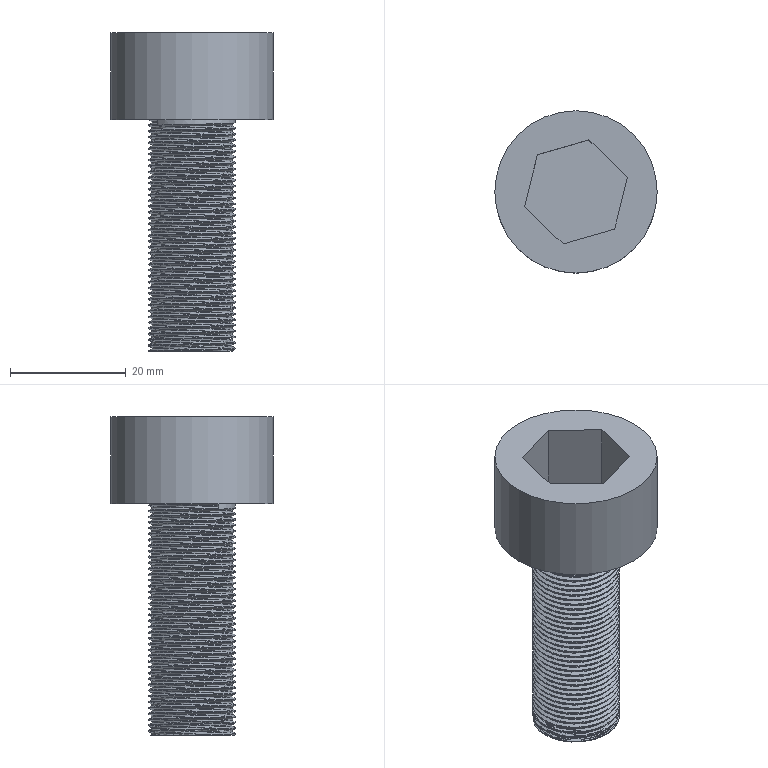Part | NX | features DATUM_CSYS 4, EXTRUDE 3, SKETCH 3, THREADS 1 | 1 solid | 18 faces | box 28 x 28 x 55 mm | volume 12823 mm3 | plane 12 | cylinder 3 | spline 3 | commonest cylinder face diameters 14 x1 15 x1 28 x1